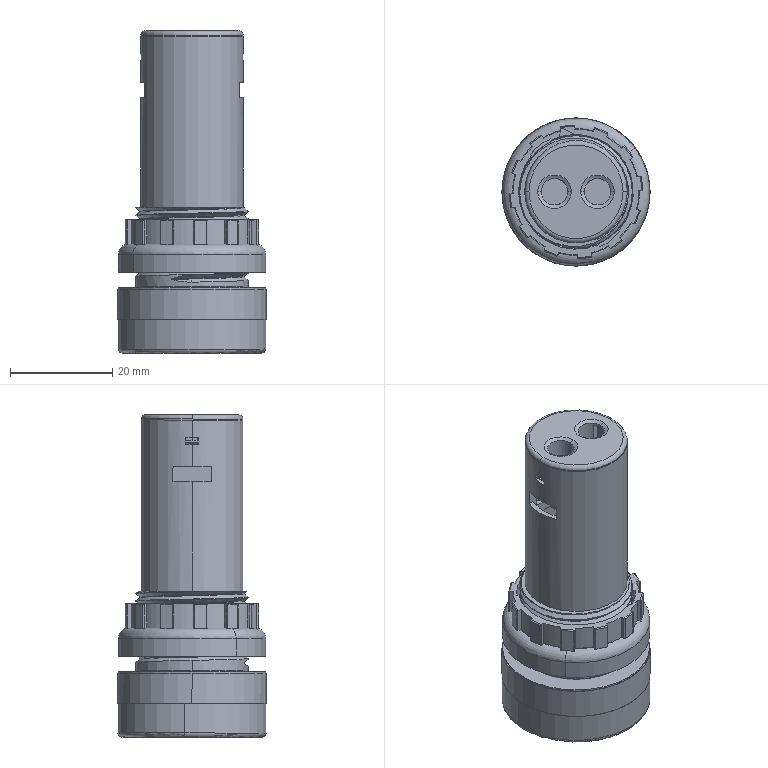Part | STEP file | Indicator Light AD17-22-AC220VW White | 5 solids | 410 faces | box 29 x 29.009 x 63.018 mm | volume 9405 mm3 | plane 192 | cylinder 170 | spline 31 | cone 9 | torus 8 | commonest cylinder face diameters 0.4 x40 22 x20 22.4 x18 24.6 x12 26.02 x11 1 x8